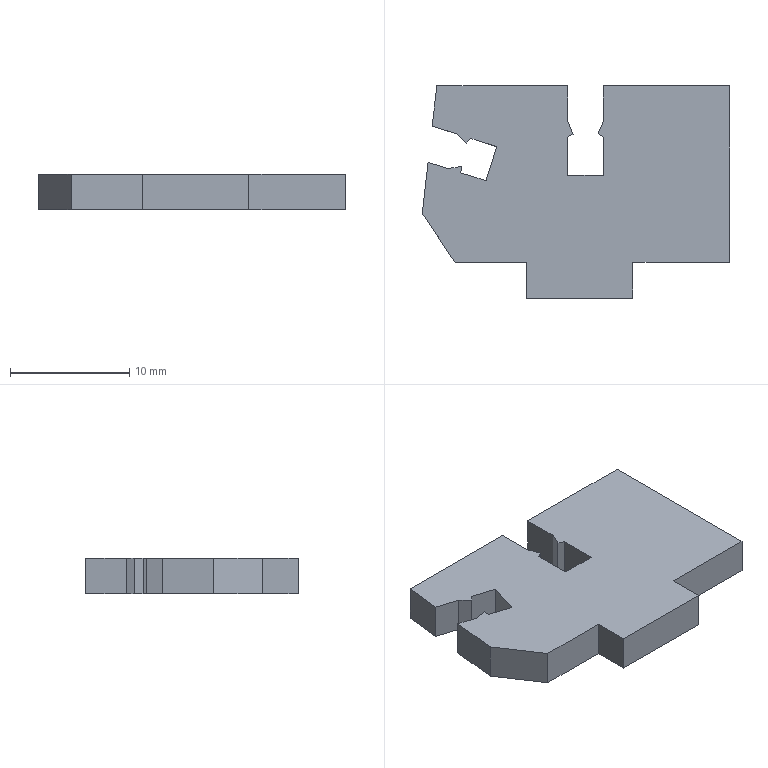Part | SolidWorks | features BaseBody 1 | 1 solid | 31 faces | box 25.767 x 17.806 x 3 mm | volume 1076 mm3 | plane 28 | spline 3
STEP:
#1=CARTESIAN_POINT('',(-24.945,11.421,-1.5));
#2=VERTEX_POINT('',#1);
#3=CARTESIAN_POINT('',(-24.55,14.81,-1.5));
#4=VERTEX_POINT('',#3);
#5=CARTESIAN_POINT('',(-24.945,11.421,-1.5));
#6=CARTESIAN_POINT('',(-24.682,13.68,-1.5));
#7=CARTESIAN_POINT('',(-24.55,14.81,-1.5));
#8=B_SPLINE_CURVE_WITH_KNOTS('',2,(#5,#6,#7),.UNSPECIFIED.,.F.,.F.,(3,3),(0.7869,0.8033),.UNSPECIFIED.);
#9=EDGE_CURVE('',#2,#4,#8,.T.);
#10=ORIENTED_EDGE('',*,*,#9,.T.);
#11=CARTESIAN_POINT('',(-13.58,14.81,-1.5));
#12=VERTEX_POINT('',#11);
#13=CARTESIAN_POINT('',(0.,14.81,-1.5));
#14=DIRECTION('',(1.,0.,0.));
#15=VECTOR('',#14,1000.);
#16=LINE('',#13,#15);
#17=EDGE_CURVE('',#4,#12,#16,.T.);
#18=ORIENTED_EDGE('',*,*,#17,.T.);
#19=CARTESIAN_POINT('',(-13.58,11.816,-1.5));
#20=VERTEX_POINT('',#19);
#21=CARTESIAN_POINT('',(-13.58,0.,-1.5));
#22=DIRECTION('',(0.,-1.,0.));
#23=VECTOR('',#22,1000.);
#24=LINE('',#21,#23);
#25=EDGE_CURVE('',#12,#20,#24,.T.);
#26=ORIENTED_EDGE('',*,*,#25,.T.);
#27=CARTESIAN_POINT('',(-13.131,10.745,-1.5));
#28=VERTEX_POINT('',#27);
#29=CARTESIAN_POINT('',(-7.343,-3.075,-1.5));
#30=DIRECTION('',(0.3863,-0.9224,0.));
#31=VECTOR('',#30,1000.);
#32=LINE('',#29,#31);
#33=EDGE_CURVE('',#20,#28,#32,.T.);
#34=ORIENTED_EDGE('',*,*,#33,.T.);
#35=CARTESIAN_POINT('',(-13.581,10.515,-1.5));
#36=VERTEX_POINT('',#35);
#37=CARTESIAN_POINT('',(-7.082,13.841,-1.5));
#38=DIRECTION('',(-0.8902,-0.4555,0.));
#39=VECTOR('',#38,1000.);
#40=LINE('',#37,#39);
#41=EDGE_CURVE('',#28,#36,#40,.T.);
#42=ORIENTED_EDGE('',*,*,#41,.T.);
#43=CARTESIAN_POINT('',(-13.583,7.301,-1.5));
#44=VERTEX_POINT('',#43);
#45=CARTESIAN_POINT('',(-13.586,0.006341,-1.5));
#46=DIRECTION('',(-0.0004667,-1.,0.));
#47=VECTOR('',#46,1000.);
#48=LINE('',#45,#47);
#49=EDGE_CURVE('',#36,#44,#48,.T.);
#50=ORIENTED_EDGE('',*,*,#49,.T.);
#51=CARTESIAN_POINT('',(-10.586,7.301,-1.5));
#52=VERTEX_POINT('',#51);
#53=CARTESIAN_POINT('',(0.,7.301,-1.5));
#54=DIRECTION('',(1.,0.,0.));
#55=VECTOR('',#54,1000.);
#56=LINE('',#53,#55);
#57=EDGE_CURVE('',#44,#52,#56,.T.);
#58=ORIENTED_EDGE('',*,*,#57,.T.);
#59=CARTESIAN_POINT('',(-10.586,10.515,-1.5));
#60=VERTEX_POINT('',#59);
#61=CARTESIAN_POINT('',(-10.586,0.,-1.5));
#62=DIRECTION('',(0.,1.,0.));
#63=VECTOR('',#62,1000.);
#64=LINE('',#61,#63);
#65=EDGE_CURVE('',#52,#60,#64,.T.);
#66=ORIENTED_EDGE('',*,*,#65,.T.);
#67=CARTESIAN_POINT('',(-11.036,10.778,-1.5));
#68=VERTEX_POINT('',#67);
#69=CARTESIAN_POINT('',(1.886,3.227,-1.5));
#70=DIRECTION('',(-0.8634,0.5045,0.));
#71=VECTOR('',#70,1000.);
#72=LINE('',#69,#71);
#73=EDGE_CURVE('',#60,#68,#72,.T.);
#74=ORIENTED_EDGE('',*,*,#73,.T.);
#75=CARTESIAN_POINT('',(-10.586,11.816,-1.5));
#76=VERTEX_POINT('',#75);
#77=CARTESIAN_POINT('',(-13.223,5.739,-1.5));
#78=DIRECTION('',(0.3981,0.9173,0.));
#79=VECTOR('',#78,1000.);
#80=LINE('',#77,#79);
#81=EDGE_CURVE('',#68,#76,#80,.T.);
#82=ORIENTED_EDGE('',*,*,#81,.T.);
#83=CARTESIAN_POINT('',(-10.588,14.81,-1.5));
#84=VERTEX_POINT('',#83);
#85=CARTESIAN_POINT('',(-10.578,-0.007066,-1.5));
#86=DIRECTION('',(-0.000668,1.,0.));
#87=VECTOR('',#86,1000.);
#88=LINE('',#85,#87);
#89=EDGE_CURVE('',#76,#84,#88,.T.);
#90=ORIENTED_EDGE('',*,*,#89,.T.);
#91=CARTESIAN_POINT('',(0.,14.81,-1.5));
#92=VERTEX_POINT('',#91);
#93=CARTESIAN_POINT('',(0.,14.81,-1.5));
#94=DIRECTION('',(1.,0.,0.));
#95=VECTOR('',#94,1000.);
#96=LINE('',#93,#95);
#97=EDGE_CURVE('',#84,#92,#96,.T.);
#98=ORIENTED_EDGE('',*,*,#97,.T.);
#99=CARTESIAN_POINT('',(0.,0.,-1.5));
#100=VERTEX_POINT('',#99);
#101=CARTESIAN_POINT('',(0.,0.,-1.5));
#102=DIRECTION('',(0.,-1.,0.));
#103=VECTOR('',#102,1000.);
#104=LINE('',#101,#103);
#105=EDGE_CURVE('',#92,#100,#104,.T.);
#106=ORIENTED_EDGE('',*,*,#105,.T.);
#107=CARTESIAN_POINT('',(-8.113,0.,-1.5));
#108=VERTEX_POINT('',#107);
#109=CARTESIAN_POINT('',(0.,0.,-1.5));
#110=DIRECTION('',(-1.,0.,0.));
#111=VECTOR('',#110,1000.);
#112=LINE('',#109,#111);
#113=EDGE_CURVE('',#100,#108,#112,.T.);
#114=ORIENTED_EDGE('',*,*,#113,.T.);
#115=CARTESIAN_POINT('',(-8.113,-2.996,-1.5));
#116=VERTEX_POINT('',#115);
#117=CARTESIAN_POINT('',(-8.113,0.,-1.5));
#118=DIRECTION('',(0.,1.,0.));
#119=VECTOR('',#118,1000.);
#120=LINE('',#117,#119);
#121=EDGE_CURVE('',#116,#108,#120,.T.);
#122=ORIENTED_EDGE('',*,*,#121,.F.);
#123=CARTESIAN_POINT('',(-17.009,-2.996,-1.5));
#124=VERTEX_POINT('',#123);
#125=CARTESIAN_POINT('',(0.,-2.996,-1.5));
#126=DIRECTION('',(-1.,0.,0.));
#127=VECTOR('',#126,1000.);
#128=LINE('',#125,#127);
#129=EDGE_CURVE('',#116,#124,#128,.T.);
#130=ORIENTED_EDGE('',*,*,#129,.T.);
#131=CARTESIAN_POINT('',(-17.009,0.,-1.5));
#132=VERTEX_POINT('',#131);
#133=CARTESIAN_POINT('',(-17.009,0.,-1.5));
#134=DIRECTION('',(0.,1.,0.));
#135=VECTOR('',#134,1000.);
#136=LINE('',#133,#135);
#137=EDGE_CURVE('',#124,#132,#136,.T.);
#138=ORIENTED_EDGE('',*,*,#137,.T.);
#139=CARTESIAN_POINT('',(-23.02,0.,-1.5));
#140=VERTEX_POINT('',#139);
#141=CARTESIAN_POINT('',(0.,0.,-1.5));
#142=DIRECTION('',(-1.,0.,0.));
#143=VECTOR('',#142,1000.);
#144=LINE('',#141,#143);
#145=EDGE_CURVE('',#132,#140,#144,.T.);
#146=ORIENTED_EDGE('',*,*,#145,.T.);
#147=CARTESIAN_POINT('',(-25.767,4.099,-1.5));
#148=VERTEX_POINT('',#147);
#149=CARTESIAN_POINT('',(-23.02,0.,-1.5));
#150=CARTESIAN_POINT('',(-23.935,1.367,-1.5));
#151=CARTESIAN_POINT('',(-24.85,2.732,-1.5));
#152=CARTESIAN_POINT('',(-25.767,4.099,-1.5));
#153=B_SPLINE_CURVE_WITH_KNOTS('',3,(#149,#150,#151,#152),.UNSPECIFIED.,.F.,.F.,(4,4),(0.6066,0.623),.UNSPECIFIED.);
#154=EDGE_CURVE('',#140,#148,#153,.T.);
#155=ORIENTED_EDGE('',*,*,#154,.T.);
#156=CARTESIAN_POINT('',(-25.29,8.389,-1.5));
#157=VERTEX_POINT('',#156);
#158=CARTESIAN_POINT('',(-25.767,4.099,-1.5));
#159=CARTESIAN_POINT('',(-25.607,5.531,-1.5));
#160=CARTESIAN_POINT('',(-25.29,8.389,-1.5));
#161=B_SPLINE_CURVE_WITH_KNOTS('',2,(#158,#159,#160),.UNSPECIFIED.,.F.,.F.,(3,3),(0.623,0.6393),.UNSPECIFIED.);
#162=EDGE_CURVE('',#148,#157,#161,.T.);
#163=ORIENTED_EDGE('',*,*,#162,.T.);
#164=CARTESIAN_POINT('',(-23.637,7.866,-1.5));
#165=VERTEX_POINT('',#164);
#166=CARTESIAN_POINT('',(0.1104,0.3489,-1.5));
#167=DIRECTION('',(0.9534,-0.3018,0.));
#168=VECTOR('',#167,1000.);
#169=LINE('',#166,#168);
#170=EDGE_CURVE('',#157,#165,#169,.T.);
#171=ORIENTED_EDGE('',*,*,#170,.T.);
#172=CARTESIAN_POINT('',(-22.501,8.049,-1.5));
#173=VERTEX_POINT('',#172);
#174=CARTESIAN_POINT('',(-1.84,11.387,-1.5));
#175=DIRECTION('',(0.9872,0.1595,0.));
#176=VECTOR('',#175,1000.);
#177=LINE('',#174,#176);
#178=EDGE_CURVE('',#165,#173,#177,.T.);
#179=ORIENTED_EDGE('',*,*,#178,.T.);
#180=CARTESIAN_POINT('',(-22.532,7.516,-1.5));
#181=VERTEX_POINT('',#180);
#182=CARTESIAN_POINT('',(-22.89,1.325,-1.5));
#183=DIRECTION('',(-0.05779,-0.9983,0.));
#184=VECTOR('',#183,1000.);
#185=LINE('',#182,#184);
#186=EDGE_CURVE('',#173,#181,#185,.T.);
#187=ORIENTED_EDGE('',*,*,#186,.T.);
#188=CARTESIAN_POINT('',(-20.425,6.852,-1.5));
#189=VERTEX_POINT('',#188);
#190=CARTESIAN_POINT('',(0.1206,0.3831,-1.5));
#191=DIRECTION('',(0.9538,-0.3003,0.));
#192=VECTOR('',#191,1000.);
#193=LINE('',#190,#192);
#194=EDGE_CURVE('',#181,#189,#193,.T.);
#195=ORIENTED_EDGE('',*,*,#194,.T.);
#196=CARTESIAN_POINT('',(-19.523,9.709,-1.5));
#197=VERTEX_POINT('',#196);
#198=CARTESIAN_POINT('',(-20.541,6.485,-1.5));
#199=DIRECTION('',(0.3011,0.9536,0.));
#200=VECTOR('',#199,1000.);
#201=LINE('',#198,#200);
#202=EDGE_CURVE('',#189,#197,#201,.T.);
#203=ORIENTED_EDGE('',*,*,#202,.T.);
#204=CARTESIAN_POINT('',(-21.692,10.394,-1.5));
#205=VERTEX_POINT('',#204);
#206=CARTESIAN_POINT('',(1.019,3.229,-1.5));
#207=DIRECTION('',(-0.9537,0.3009,0.));
#208=VECTOR('',#207,1000.);
#209=LINE('',#206,#208);
#210=EDGE_CURVE('',#197,#205,#209,.T.);
#211=ORIENTED_EDGE('',*,*,#210,.T.);
#212=CARTESIAN_POINT('',(-22.05,10.009,-1.5));
#213=VERTEX_POINT('',#212);
#214=CARTESIAN_POINT('',(-16.776,15.659,-1.5));
#215=DIRECTION('',(-0.6824,-0.731,0.));
#216=VECTOR('',#215,1000.);
#217=LINE('',#214,#216);
#218=EDGE_CURVE('',#205,#213,#217,.T.);
#219=ORIENTED_EDGE('',*,*,#218,.T.);
#220=CARTESIAN_POINT('',(-22.83,10.752,-1.5));
#221=VERTEX_POINT('',#220);
#222=CARTESIAN_POINT('',(-5.502,-5.77,-1.5));
#223=DIRECTION('',(-0.7237,0.6901,0.));
#224=VECTOR('',#223,1000.);
#225=LINE('',#222,#224);
#226=EDGE_CURVE('',#213,#221,#225,.T.);
#227=ORIENTED_EDGE('',*,*,#226,.T.);
#228=CARTESIAN_POINT('',(1.015,3.211,-1.5));
#229=DIRECTION('',(-0.9535,0.3015,0.));
#230=VECTOR('',#229,1000.);
#231=LINE('',#228,#230);
#232=EDGE_CURVE('',#221,#2,#231,.T.);
#233=ORIENTED_EDGE('',*,*,#232,.T.);
#234=EDGE_LOOP('',(#10,#18,#26,#34,#42,#50,#58,#66,#74,#82,#90,#98,#106,#114,#122,#130,#138,#146,#155,#163,#171,#179,#187,#195,#203,#211,#219,#227,#233));
#235=FACE_OUTER_BOUND('',#234,.T.);
#236=CARTESIAN_POINT('',(0.,0.,-1.5));
#237=DIRECTION('',(0.,0.,1.));
#238=DIRECTION('',(1.,0.,0.));
#239=AXIS2_PLACEMENT_3D('',#236,#237,#238);
#240=PLANE('',#239);
#241=ADVANCED_FACE('',(#235),#240,.F.);
#242=CARTESIAN_POINT('',(-24.945,11.421,1.5));
#243=VERTEX_POINT('',#242);
#244=CARTESIAN_POINT('',(-24.55,14.81,1.5));
#245=VERTEX_POINT('',#244);
#246=CARTESIAN_POINT('',(-24.945,11.421,1.5));
#247=CARTESIAN_POINT('',(-24.682,13.68,1.5));
#248=CARTESIAN_POINT('',(-24.55,14.81,1.5));
#249=B_SPLINE_CURVE_WITH_KNOTS('',2,(#246,#247,#248),.UNSPECIFIED.,.F.,.F.,(3,3),(0.7869,0.8033),.UNSPECIFIED.);
#250=EDGE_CURVE('',#243,#245,#249,.T.);
#251=ORIENTED_EDGE('',*,*,#250,.F.);
#252=CARTESIAN_POINT('',(-22.83,10.752,1.5));
#253=VERTEX_POINT('',#252);
#254=CARTESIAN_POINT('',(1.015,3.211,1.5));
#255=DIRECTION('',(-0.9535,0.3015,0.));
#256=VECTOR('',#255,1000.);
#257=LINE('',#254,#256);
#258=EDGE_CURVE('',#253,#243,#257,.T.);
#259=ORIENTED_EDGE('',*,*,#258,.F.);
#260=CARTESIAN_POINT('',(-22.05,10.009,1.5));
#261=VERTEX_POINT('',#260);
#262=CARTESIAN_POINT('',(-5.502,-5.77,1.5));
#263=DIRECTION('',(-0.7237,0.6901,0.));
#264=VECTOR('',#263,1000.);
#265=LINE('',#262,#264);
#266=EDGE_CURVE('',#261,#253,#265,.T.);
#267=ORIENTED_EDGE('',*,*,#266,.F.);
#268=CARTESIAN_POINT('',(-21.692,10.394,1.5));
#269=VERTEX_POINT('',#268);
#270=CARTESIAN_POINT('',(-16.776,15.659,1.5));
#271=DIRECTION('',(-0.6824,-0.731,0.));
#272=VECTOR('',#271,1000.);
#273=LINE('',#270,#272);
#274=EDGE_CURVE('',#269,#261,#273,.T.);
#275=ORIENTED_EDGE('',*,*,#274,.F.);
#276=CARTESIAN_POINT('',(-19.523,9.709,1.5));
#277=VERTEX_POINT('',#276);
#278=CARTESIAN_POINT('',(1.019,3.229,1.5));
#279=DIRECTION('',(-0.9537,0.3009,0.));
#280=VECTOR('',#279,1000.);
#281=LINE('',#278,#280);
#282=EDGE_CURVE('',#277,#269,#281,.T.);
#283=ORIENTED_EDGE('',*,*,#282,.F.);
#284=CARTESIAN_POINT('',(-20.425,6.852,1.5));
#285=VERTEX_POINT('',#284);
#286=CARTESIAN_POINT('',(-20.541,6.485,1.5));
#287=DIRECTION('',(0.3011,0.9536,0.));
#288=VECTOR('',#287,1000.);
#289=LINE('',#286,#288);
#290=EDGE_CURVE('',#285,#277,#289,.T.);
#291=ORIENTED_EDGE('',*,*,#290,.F.);
#292=CARTESIAN_POINT('',(-22.532,7.516,1.5));
#293=VERTEX_POINT('',#292);
#294=CARTESIAN_POINT('',(0.1206,0.3831,1.5));
#295=DIRECTION('',(0.9538,-0.3003,0.));
#296=VECTOR('',#295,1000.);
#297=LINE('',#294,#296);
#298=EDGE_CURVE('',#293,#285,#297,.T.);
#299=ORIENTED_EDGE('',*,*,#298,.F.);
#300=CARTESIAN_POINT('',(-22.501,8.049,1.5));
#301=VERTEX_POINT('',#300);
#302=CARTESIAN_POINT('',(-22.89,1.325,1.5));
#303=DIRECTION('',(-0.05779,-0.9983,0.));
#304=VECTOR('',#303,1000.);
#305=LINE('',#302,#304);
#306=EDGE_CURVE('',#301,#293,#305,.T.);
#307=ORIENTED_EDGE('',*,*,#306,.F.);
#308=CARTESIAN_POINT('',(-23.637,7.866,1.5));
#309=VERTEX_POINT('',#308);
#310=CARTESIAN_POINT('',(-1.84,11.387,1.5));
#311=DIRECTION('',(0.9872,0.1595,0.));
#312=VECTOR('',#311,1000.);
#313=LINE('',#310,#312);
#314=EDGE_CURVE('',#309,#301,#313,.T.);
#315=ORIENTED_EDGE('',*,*,#314,.F.);
#316=CARTESIAN_POINT('',(-25.29,8.389,1.5));
#317=VERTEX_POINT('',#316);
#318=CARTESIAN_POINT('',(0.1104,0.3489,1.5));
#319=DIRECTION('',(0.9534,-0.3018,0.));
#320=VECTOR('',#319,1000.);
#321=LINE('',#318,#320);
#322=EDGE_CURVE('',#317,#309,#321,.T.);
#323=ORIENTED_EDGE('',*,*,#322,.F.);
#324=CARTESIAN_POINT('',(-25.767,4.099,1.5));
#325=VERTEX_POINT('',#324);
#326=CARTESIAN_POINT('',(-25.767,4.099,1.5));
#327=CARTESIAN_POINT('',(-25.607,5.531,1.5));
#328=CARTESIAN_POINT('',(-25.29,8.389,1.5));
#329=B_SPLINE_CURVE_WITH_KNOTS('',2,(#326,#327,#328),.UNSPECIFIED.,.F.,.F.,(3,3),(0.623,0.6393),.UNSPECIFIED.);
#330=EDGE_CURVE('',#325,#317,#329,.T.);
#331=ORIENTED_EDGE('',*,*,#330,.F.);
#332=CARTESIAN_POINT('',(-23.02,0.,1.5));
#333=VERTEX_POINT('',#332);
#334=CARTESIAN_POINT('',(-23.02,0.,1.5));
#335=CARTESIAN_POINT('',(-23.935,1.367,1.5));
#336=CARTESIAN_POINT('',(-24.85,2.732,1.5));
#337=CARTESIAN_POINT('',(-25.767,4.099,1.5));
#338=B_SPLINE_CURVE_WITH_KNOTS('',3,(#334,#335,#336,#337),.UNSPECIFIED.,.F.,.F.,(4,4),(0.6066,0.623),.UNSPECIFIED.);
#339=EDGE_CURVE('',#333,#325,#338,.T.);
#340=ORIENTED_EDGE('',*,*,#339,.F.);
#341=CARTESIAN_POINT('',(-17.009,0.,1.5));
#342=VERTEX_POINT('',#341);
#343=CARTESIAN_POINT('',(0.,0.,1.5));
#344=DIRECTION('',(-1.,0.,0.));
#345=VECTOR('',#344,1000.);
#346=LINE('',#343,#345);
#347=EDGE_CURVE('',#342,#333,#346,.T.);
#348=ORIENTED_EDGE('',*,*,#347,.F.);
#349=CARTESIAN_POINT('',(-17.009,-2.996,1.5));
#350=VERTEX_POINT('',#349);
#351=CARTESIAN_POINT('',(-17.009,0.,1.5));
#352=DIRECTION('',(0.,1.,0.));
#353=VECTOR('',#352,1000.);
#354=LINE('',#351,#353);
#355=EDGE_CURVE('',#350,#342,#354,.T.);
#356=ORIENTED_EDGE('',*,*,#355,.F.);
#357=CARTESIAN_POINT('',(-8.113,-2.996,1.5));
#358=VERTEX_POINT('',#357);
#359=CARTESIAN_POINT('',(0.,-2.996,1.5));
#360=DIRECTION('',(-1.,0.,0.));
#361=VECTOR('',#360,1000.);
#362=LINE('',#359,#361);
#363=EDGE_CURVE('',#358,#350,#362,.T.);
#364=ORIENTED_EDGE('',*,*,#363,.F.);
#365=CARTESIAN_POINT('',(-8.113,0.,1.5));
#366=VERTEX_POINT('',#365);
#367=CARTESIAN_POINT('',(-8.113,0.,1.5));
#368=DIRECTION('',(0.,1.,0.));
#369=VECTOR('',#368,1000.);
#370=LINE('',#367,#369);
#371=EDGE_CURVE('',#358,#366,#370,.T.);
#372=ORIENTED_EDGE('',*,*,#371,.T.);
#373=CARTESIAN_POINT('',(0.,0.,1.5));
#374=VERTEX_POINT('',#373);
#375=CARTESIAN_POINT('',(0.,0.,1.5));
#376=DIRECTION('',(-1.,0.,0.));
#377=VECTOR('',#376,1000.);
#378=LINE('',#375,#377);
#379=EDGE_CURVE('',#374,#366,#378,.T.);
#380=ORIENTED_EDGE('',*,*,#379,.F.);
#381=CARTESIAN_POINT('',(0.,14.81,1.5));
#382=VERTEX_POINT('',#381);
#383=CARTESIAN_POINT('',(0.,0.,1.5));
#384=DIRECTION('',(0.,-1.,0.));
#385=VECTOR('',#384,1000.);
#386=LINE('',#383,#385);
#387=EDGE_CURVE('',#382,#374,#386,.T.);
#388=ORIENTED_EDGE('',*,*,#387,.F.);
#389=CARTESIAN_POINT('',(-10.588,14.81,1.5));
#390=VERTEX_POINT('',#389);
#391=CARTESIAN_POINT('',(0.,14.81,1.5));
#392=DIRECTION('',(1.,0.,0.));
#393=VECTOR('',#392,1000.);
#394=LINE('',#391,#393);
#395=EDGE_CURVE('',#390,#382,#394,.T.);
#396=ORIENTED_EDGE('',*,*,#395,.F.);
#397=CARTESIAN_POINT('',(-10.586,11.816,1.5));
#398=VERTEX_POINT('',#397);
#399=CARTESIAN_POINT('',(-10.578,-0.007066,1.5));
#400=DIRECTION('',(-0.000668,1.,0.));
#401=VECTOR('',#400,1000.);
#402=LINE('',#399,#401);
#403=EDGE_CURVE('',#398,#390,#402,.T.);
#404=ORIENTED_EDGE('',*,*,#403,.F.);
#405=CARTESIAN_POINT('',(-11.036,10.778,1.5));
#406=VERTEX_POINT('',#405);
#407=CARTESIAN_POINT('',(-13.223,5.739,1.5));
#408=DIRECTION('',(0.3981,0.9173,0.));
#409=VECTOR('',#408,1000.);
#410=LINE('',#407,#409);
#411=EDGE_CURVE('',#406,#398,#410,.T.);
#412=ORIENTED_EDGE('',*,*,#411,.F.);
#413=CARTESIAN_POINT('',(-10.586,10.515,1.5));
#414=VERTEX_POINT('',#413);
#415=CARTESIAN_POINT('',(1.886,3.227,1.5));
#416=DIRECTION('',(-0.8634,0.5045,0.));
#417=VECTOR('',#416,1000.);
#418=LINE('',#415,#417);
#419=EDGE_CURVE('',#414,#406,#418,.T.);
#420=ORIENTED_EDGE('',*,*,#419,.F.);
#421=CARTESIAN_POINT('',(-10.586,7.301,1.5));
#422=VERTEX_POINT('',#421);
#423=CARTESIAN_POINT('',(-10.586,0.,1.5));
#424=DIRECTION('',(0.,1.,0.));
#425=VECTOR('',#424,1000.);
#426=LINE('',#423,#425);
#427=EDGE_CURVE('',#422,#414,#426,.T.);
#428=ORIENTED_EDGE('',*,*,#427,.F.);
#429=CARTESIAN_POINT('',(-13.583,7.301,1.5));
#430=VERTEX_POINT('',#429);
#431=CARTESIAN_POINT('',(0.,7.301,1.5));
#432=DIRECTION('',(1.,0.,0.));
#433=VECTOR('',#432,1000.);
#434=LINE('',#431,#433);
#435=EDGE_CURVE('',#430,#422,#434,.T.);
#436=ORIENTED_EDGE('',*,*,#435,.F.);
#437=CARTESIAN_POINT('',(-13.581,10.515,1.5));
#438=VERTEX_POINT('',#437);
#439=CARTESIAN_POINT('',(-13.586,0.006341,1.5));
#440=DIRECTION('',(-0.0004667,-1.,0.));
#441=VECTOR('',#440,1000.);
#442=LINE('',#439,#441);
#443=EDGE_CURVE('',#438,#430,#442,.T.);
#444=ORIENTED_EDGE('',*,*,#443,.F.);
#445=CARTESIAN_POINT('',(-13.131,10.745,1.5));
#446=VERTEX_POINT('',#445);
#447=CARTESIAN_POINT('',(-7.082,13.841,1.5));
#448=DIRECTION('',(-0.8902,-0.4555,0.));
#449=VECTOR('',#448,1000.);
#450=LINE('',#447,#449);
#451=EDGE_CURVE('',#446,#438,#450,.T.);
#452=ORIENTED_EDGE('',*,*,#451,.F.);
#453=CARTESIAN_POINT('',(-13.58,11.816,1.5));
#454=VERTEX_POINT('',#453);
#455=CARTESIAN_POINT('',(-7.343,-3.075,1.5));
#456=DIRECTION('',(0.3863,-0.9224,0.));
#457=VECTOR('',#456,1000.);
#458=LINE('',#455,#457);
#459=EDGE_CURVE('',#454,#446,#458,.T.);
#460=ORIENTED_EDGE('',*,*,#459,.F.);
#461=CARTESIAN_POINT('',(-13.58,14.81,1.5));
#462=VERTEX_POINT('',#461);
#463=CARTESIAN_POINT('',(-13.58,0.,1.5));
#464=DIRECTION('',(0.,-1.,0.));
#465=VECTOR('',#464,1000.);
#466=LINE('',#463,#465);
#467=EDGE_CURVE('',#462,#454,#466,.T.);
#468=ORIENTED_EDGE('',*,*,#467,.F.);
#469=CARTESIAN_POINT('',(0.,14.81,1.5));
#470=DIRECTION('',(1.,0.,0.));
#471=VECTOR('',#470,1000.);
#472=LINE('',#469,#471);
#473=EDGE_CURVE('',#245,#462,#472,.T.);
#474=ORIENTED_EDGE('',*,*,#473,.F.);
#475=EDGE_LOOP('',(#251,#259,#267,#275,#283,#291,#299,#307,#315,#323,#331,#340,#348,#356,#364,#372,#380,#388,#396,#404,#412,#420,#428,#436,#444,#452,#460,#468,#474));
#476=FACE_OUTER_BOUND('',#475,.T.);
#477=CARTESIAN_POINT('',(0.,0.,1.5));
#478=DIRECTION('',(0.,0.,1.));
#479=DIRECTION('',(1.,0.,0.));
#480=AXIS2_PLACEMENT_3D('',#477,#478,#479);
#481=PLANE('',#480);
#482=ADVANCED_FACE('',(#476),#481,.T.);
#483=ORIENTED_EDGE('',*,*,#17,.F.);
#484=CARTESIAN_POINT('',(-24.55,14.81,1.5));
#485=DIRECTION('',(0.,0.,-1.));
#486=VECTOR('',#485,1000.);
#487=LINE('',#484,#486);
#488=EDGE_CURVE('',#245,#4,#487,.T.);
#489=ORIENTED_EDGE('',*,*,#488,.F.);
#490=ORIENTED_EDGE('',*,*,#473,.T.);
#491=CARTESIAN_POINT('',(-13.58,14.81,1.5));
#492=DIRECTION('',(0.,0.,-1.));
#493=VECTOR('',#492,1000.);
#494=LINE('',#491,#493);
#495=EDGE_CURVE('',#462,#12,#494,.T.);
#496=ORIENTED_EDGE('',*,*,#495,.T.);
#497=EDGE_LOOP('',(#483,#489,#490,#496));
#498=FACE_OUTER_BOUND('',#497,.T.);
#499=CARTESIAN_POINT('',(0.,14.81,1.5));
#500=DIRECTION('',(0.,1.,0.));
#501=DIRECTION('',(1.,0.,0.));
#502=AXIS2_PLACEMENT_3D('',#499,#500,#501);
#503=PLANE('',#502);
#504=ADVANCED_FACE('',(#498),#503,.T.);
#505=ORIENTED_EDGE('',*,*,#25,.F.);
#506=ORIENTED_EDGE('',*,*,#495,.F.);
#507=ORIENTED_EDGE('',*,*,#467,.T.);
#508=CARTESIAN_POINT('',(-13.58,11.816,1.5));
#509=DIRECTION('',(0.,0.,-1.));
#510=VECTOR('',#509,1000.);
#511=LINE('',#508,#510);
#512=EDGE_CURVE('',#454,#20,#511,.T.);
#513=ORIENTED_EDGE('',*,*,#512,.T.);
#514=EDGE_LOOP('',(#505,#506,#507,#513));
#515=FACE_OUTER_BOUND('',#514,.T.);
#516=CARTESIAN_POINT('',(-13.58,0.,1.5));
#517=DIRECTION('',(1.,0.,0.));
#518=DIRECTION('',(0.,1.,0.));
#519=AXIS2_PLACEMENT_3D('',#516,#517,#518);
#520=PLANE('',#519);
#521=ADVANCED_FACE('',(#515),#520,.T.);
#522=ORIENTED_EDGE('',*,*,#33,.F.);
#523=ORIENTED_EDGE('',*,*,#512,.F.);
#524=ORIENTED_EDGE('',*,*,#459,.T.);
#525=CARTESIAN_POINT('',(-13.131,10.745,1.5));
#526=DIRECTION('',(0.,0.,-1.));
#527=VECTOR('',#526,1000.);
#528=LINE('',#525,#527);
#529=EDGE_CURVE('',#446,#28,#528,.T.);
#530=ORIENTED_EDGE('',*,*,#529,.T.);
#531=EDGE_LOOP('',(#522,#523,#524,#530));
#532=FACE_OUTER_BOUND('',#531,.T.);
#533=CARTESIAN_POINT('',(-7.343,-3.075,1.5));
#534=DIRECTION('',(0.9224,0.3863,0.));
#535=DIRECTION('',(0.,0.,-1.));
#536=AXIS2_PLACEMENT_3D('',#533,#534,#535);
#537=PLANE('',#536);
#538=ADVANCED_FACE('',(#532),#537,.T.);
#539=ORIENTED_EDGE('',*,*,#41,.F.);
#540=ORIENTED_EDGE('',*,*,#529,.F.);
#541=ORIENTED_EDGE('',*,*,#451,.T.);
#542=CARTESIAN_POINT('',(-13.581,10.515,1.5));
#543=DIRECTION('',(0.,0.,-1.));
#544=VECTOR('',#543,1000.);
#545=LINE('',#542,#544);
#546=EDGE_CURVE('',#438,#36,#545,.T.);
#547=ORIENTED_EDGE('',*,*,#546,.T.);
#548=EDGE_LOOP('',(#539,#540,#541,#547));
#549=FACE_OUTER_BOUND('',#548,.T.);
#550=CARTESIAN_POINT('',(-7.082,13.841,1.5));
#551=DIRECTION('',(0.4555,-0.8902,0.));
#552=DIRECTION('',(0.,0.,-1.));
#553=AXIS2_PLACEMENT_3D('',#550,#551,#552);
#554=PLANE('',#553);
#555=ADVANCED_FACE('',(#549),#554,.T.);
#556=ORIENTED_EDGE('',*,*,#49,.F.);
#557=ORIENTED_EDGE('',*,*,#546,.F.);
#558=ORIENTED_EDGE('',*,*,#443,.T.);
#559=CARTESIAN_POINT('',(-13.583,7.301,1.5));
#560=DIRECTION('',(0.,0.,-1.));
#561=VECTOR('',#560,1000.);
#562=LINE('',#559,#561);
#563=EDGE_CURVE('',#430,#44,#562,.T.);
#564=ORIENTED_EDGE('',*,*,#563,.T.);
#565=EDGE_LOOP('',(#556,#557,#558,#564));
#566=FACE_OUTER_BOUND('',#565,.T.);
#567=CARTESIAN_POINT('',(-13.586,0.006341,1.5));
#568=DIRECTION('',(1.,-0.0004667,0.));
#569=DIRECTION('',(0.,0.,-1.));
#570=AXIS2_PLACEMENT_3D('',#567,#568,#569);
#571=PLANE('',#570);
#572=ADVANCED_FACE('',(#566),#571,.T.);
#573=ORIENTED_EDGE('',*,*,#57,.F.);
#574=ORIENTED_EDGE('',*,*,#563,.F.);
#575=ORIENTED_EDGE('',*,*,#435,.T.);
#576=CARTESIAN_POINT('',(-10.586,7.301,1.5));
#577=DIRECTION('',(0.,0.,-1.));
#578=VECTOR('',#577,1000.);
#579=LINE('',#576,#578);
#580=EDGE_CURVE('',#422,#52,#579,.T.);
#581=ORIENTED_EDGE('',*,*,#580,.T.);
#582=EDGE_LOOP('',(#573,#574,#575,#581));
#583=FACE_OUTER_BOUND('',#582,.T.);
#584=CARTESIAN_POINT('',(0.,7.301,1.5));
#585=DIRECTION('',(0.,1.,0.));
#586=DIRECTION('',(1.,0.,0.));
#587=AXIS2_PLACEMENT_3D('',#584,#585,#586);
#588=PLANE('',#587);
#589=ADVANCED_FACE('',(#583),#588,.T.);
#590=ORIENTED_EDGE('',*,*,#65,.F.);
#591=ORIENTED_EDGE('',*,*,#580,.F.);
#592=ORIENTED_EDGE('',*,*,#427,.T.);
#593=CARTESIAN_POINT('',(-10.586,10.515,1.5));
#594=DIRECTION('',(0.,0.,-1.));
#595=VECTOR('',#594,1000.);
#596=LINE('',#593,#595);
#597=EDGE_CURVE('',#414,#60,#596,.T.);
#598=ORIENTED_EDGE('',*,*,#597,.T.);
#599=EDGE_LOOP('',(#590,#591,#592,#598));
#600=FACE_OUTER_BOUND('',#599,.T.);
#601=CARTESIAN_POINT('',(-10.586,0.,1.5));
#602=DIRECTION('',(-1.,0.,0.));
#603=DIRECTION('',(0.,0.,1.));
#604=AXIS2_PLACEMENT_3D('',#601,#602,#603);
#605=PLANE('',#604);
#606=ADVANCED_FACE('',(#600),#605,.T.);
#607=ORIENTED_EDGE('',*,*,#73,.F.);
#608=ORIENTED_EDGE('',*,*,#597,.F.);
#609=ORIENTED_EDGE('',*,*,#419,.T.);
#610=CARTESIAN_POINT('',(-11.036,10.778,1.5));
#611=DIRECTION('',(0.,0.,-1.));
#612=VECTOR('',#611,1000.);
#613=LINE('',#610,#612);
#614=EDGE_CURVE('',#406,#68,#613,.T.);
#615=ORIENTED_EDGE('',*,*,#614,.T.);
#616=EDGE_LOOP('',(#607,#608,#609,#615));
#617=FACE_OUTER_BOUND('',#616,.T.);
#618=CARTESIAN_POINT('',(1.886,3.227,1.5));
#619=DIRECTION('',(-0.5045,-0.8634,0.));
#620=DIRECTION('',(-0.8634,0.5045,0.));
#621=AXIS2_PLACEMENT_3D('',#618,#619,#620);
#622=PLANE('',#621);
#623=ADVANCED_FACE('',(#617),#622,.T.);
#624=ORIENTED_EDGE('',*,*,#81,.F.);
#625=ORIENTED_EDGE('',*,*,#614,.F.);
#626=ORIENTED_EDGE('',*,*,#411,.T.);
#627=CARTESIAN_POINT('',(-10.586,11.816,1.5));
#628=DIRECTION('',(0.,0.,-1.));
#629=VECTOR('',#628,1000.);
#630=LINE('',#627,#629);
#631=EDGE_CURVE('',#398,#76,#630,.T.);
#632=ORIENTED_EDGE('',*,*,#631,.T.);
#633=EDGE_LOOP('',(#624,#625,#626,#632));
#634=FACE_OUTER_BOUND('',#633,.T.);
#635=CARTESIAN_POINT('',(-13.223,5.739,1.5));
#636=DIRECTION('',(-0.9173,0.3981,0.));
#637=DIRECTION('',(0.,0.,1.));
#638=AXIS2_PLACEMENT_3D('',#635,#636,#637);
#639=PLANE('',#638);
#640=ADVANCED_FACE('',(#634),#639,.T.);
#641=ORIENTED_EDGE('',*,*,#89,.F.);
#642=ORIENTED_EDGE('',*,*,#631,.F.);
#643=ORIENTED_EDGE('',*,*,#403,.T.);
#644=CARTESIAN_POINT('',(-10.588,14.81,1.5));
#645=DIRECTION('',(0.,0.,-1.));
#646=VECTOR('',#645,1000.);
#647=LINE('',#644,#646);
#648=EDGE_CURVE('',#390,#84,#647,.T.);
#649=ORIENTED_EDGE('',*,*,#648,.T.);
#650=EDGE_LOOP('',(#641,#642,#643,#649));
#651=FACE_OUTER_BOUND('',#650,.T.);
#652=CARTESIAN_POINT('',(-10.578,-0.007066,1.5));
#653=DIRECTION('',(-1.,-0.000668,0.));
#654=DIRECTION('',(-0.000668,1.,0.));
#655=AXIS2_PLACEMENT_3D('',#652,#653,#654);
#656=PLANE('',#655);
#657=ADVANCED_FACE('',(#651),#656,.T.);
#658=ORIENTED_EDGE('',*,*,#97,.F.);
#659=ORIENTED_EDGE('',*,*,#648,.F.);
#660=ORIENTED_EDGE('',*,*,#395,.T.);
#661=CARTESIAN_POINT('',(0.,14.81,1.5));
#662=DIRECTION('',(0.,0.,-1.));
#663=VECTOR('',#662,1000.);
#664=LINE('',#661,#663);
#665=EDGE_CURVE('',#382,#92,#664,.T.);
#666=ORIENTED_EDGE('',*,*,#665,.T.);
#667=EDGE_LOOP('',(#658,#659,#660,#666));
#668=FACE_OUTER_BOUND('',#667,.T.);
#669=CARTESIAN_POINT('',(0.,14.81,1.5));
#670=DIRECTION('',(0.,1.,0.));
#671=DIRECTION('',(1.,0.,0.));
#672=AXIS2_PLACEMENT_3D('',#669,#670,#671);
#673=PLANE('',#672);
#674=ADVANCED_FACE('',(#668),#673,.T.);
#675=ORIENTED_EDGE('',*,*,#105,.F.);
#676=ORIENTED_EDGE('',*,*,#665,.F.);
#677=ORIENTED_EDGE('',*,*,#387,.T.);
#678=CARTESIAN_POINT('',(0.,0.,1.5));
#679=DIRECTION('',(0.,0.,-1.));
#680=VECTOR('',#679,1000.);
#681=LINE('',#678,#680);
#682=EDGE_CURVE('',#374,#100,#681,.T.);
#683=ORIENTED_EDGE('',*,*,#682,.T.);
#684=EDGE_LOOP('',(#675,#676,#677,#683));
#685=FACE_OUTER_BOUND('',#684,.T.);
#686=CARTESIAN_POINT('',(0.,0.,1.5));
#687=DIRECTION('',(1.,0.,0.));
#688=DIRECTION('',(0.,1.,0.));
#689=AXIS2_PLACEMENT_3D('',#686,#687,#688);
#690=PLANE('',#689);
#691=ADVANCED_FACE('',(#685),#690,.T.);
#692=ORIENTED_EDGE('',*,*,#113,.F.);
#693=ORIENTED_EDGE('',*,*,#682,.F.);
#694=ORIENTED_EDGE('',*,*,#379,.T.);
#695=CARTESIAN_POINT('',(-8.113,0.,1.5));
#696=DIRECTION('',(0.,0.,-1.));
#697=VECTOR('',#696,1000.);
#698=LINE('',#695,#697);
#699=EDGE_CURVE('',#366,#108,#698,.T.);
#700=ORIENTED_EDGE('',*,*,#699,.T.);
#701=EDGE_LOOP('',(#692,#693,#694,#700));
#702=FACE_OUTER_BOUND('',#701,.T.);
#703=CARTESIAN_POINT('',(0.,0.,1.5));
#704=DIRECTION('',(0.,-1.,0.));
#705=DIRECTION('',(0.,0.,-1.));
#706=AXIS2_PLACEMENT_3D('',#703,#704,#705);
#707=PLANE('',#706);
#708=ADVANCED_FACE('',(#702),#707,.T.);
#709=ORIENTED_EDGE('',*,*,#121,.T.);
#710=ORIENTED_EDGE('',*,*,#699,.F.);
#711=ORIENTED_EDGE('',*,*,#371,.F.);
#712=CARTESIAN_POINT('',(-8.113,-2.996,1.5));
#713=DIRECTION('',(0.,0.,-1.));
#714=VECTOR('',#713,1000.);
#715=LINE('',#712,#714);
#716=EDGE_CURVE('',#358,#116,#715,.T.);
#717=ORIENTED_EDGE('',*,*,#716,.T.);
#718=EDGE_LOOP('',(#709,#710,#711,#717));
#719=FACE_OUTER_BOUND('',#718,.T.);
#720=CARTESIAN_POINT('',(-8.113,0.,1.5));
#721=DIRECTION('',(-1.,0.,0.));
#722=DIRECTION('',(0.,0.,1.));
#723=AXIS2_PLACEMENT_3D('',#720,#721,#722);
#724=PLANE('',#723);
#725=ADVANCED_FACE('',(#719),#724,.F.);
#726=ORIENTED_EDGE('',*,*,#129,.F.);
#727=ORIENTED_EDGE('',*,*,#716,.F.);
#728=ORIENTED_EDGE('',*,*,#363,.T.);
#729=CARTESIAN_POINT('',(-17.009,-2.996,1.5));
#730=DIRECTION('',(0.,0.,-1.));
#731=VECTOR('',#730,1000.);
#732=LINE('',#729,#731);
#733=EDGE_CURVE('',#350,#124,#732,.T.);
#734=ORIENTED_EDGE('',*,*,#733,.T.);
#735=EDGE_LOOP('',(#726,#727,#728,#734));
#736=FACE_OUTER_BOUND('',#735,.T.);
#737=CARTESIAN_POINT('',(0.,-2.996,1.5));
#738=DIRECTION('',(0.,-1.,0.));
#739=DIRECTION('',(0.,0.,-1.));
#740=AXIS2_PLACEMENT_3D('',#737,#738,#739);
#741=PLANE('',#740);
#742=ADVANCED_FACE('',(#736),#741,.T.);
#743=ORIENTED_EDGE('',*,*,#137,.F.);
#744=ORIENTED_EDGE('',*,*,#733,.F.);
#745=ORIENTED_EDGE('',*,*,#355,.T.);
#746=CARTESIAN_POINT('',(-17.009,0.,1.5));
#747=DIRECTION('',(0.,0.,-1.));
#748=VECTOR('',#747,1000.);
#749=LINE('',#746,#748);
#750=EDGE_CURVE('',#342,#132,#749,.T.);
#751=ORIENTED_EDGE('',*,*,#750,.T.);
#752=EDGE_LOOP('',(#743,#744,#745,#751));
#753=FACE_OUTER_BOUND('',#752,.T.);
#754=CARTESIAN_POINT('',(-17.009,0.,1.5));
#755=DIRECTION('',(-1.,0.,0.));
#756=DIRECTION('',(0.,0.,1.));
#757=AXIS2_PLACEMENT_3D('',#754,#755,#756);
#758=PLANE('',#757);
#759=ADVANCED_FACE('',(#753),#758,.T.);
#760=ORIENTED_EDGE('',*,*,#145,.F.);
#761=ORIENTED_EDGE('',*,*,#750,.F.);
#762=ORIENTED_EDGE('',*,*,#347,.T.);
#763=CARTESIAN_POINT('',(-23.02,0.,1.5));
#764=DIRECTION('',(0.,0.,-1.));
#765=VECTOR('',#764,1000.);
#766=LINE('',#763,#765);
#767=EDGE_CURVE('',#333,#140,#766,.T.);
#768=ORIENTED_EDGE('',*,*,#767,.T.);
#769=EDGE_LOOP('',(#760,#761,#762,#768));
#770=FACE_OUTER_BOUND('',#769,.T.);
#771=CARTESIAN_POINT('',(0.,0.,1.5));
#772=DIRECTION('',(0.,-1.,0.));
#773=DIRECTION('',(0.,0.,-1.));
#774=AXIS2_PLACEMENT_3D('',#771,#772,#773);
#775=PLANE('',#774);
#776=ADVANCED_FACE('',(#770),#775,.T.);
#777=ORIENTED_EDGE('',*,*,#154,.F.);
#778=ORIENTED_EDGE('',*,*,#767,.F.);
#779=ORIENTED_EDGE('',*,*,#339,.T.);
#780=CARTESIAN_POINT('',(-25.767,4.099,1.5));
#781=DIRECTION('',(0.,0.,-1.));
#782=VECTOR('',#781,1000.);
#783=LINE('',#780,#782);
#784=EDGE_CURVE('',#325,#148,#783,.T.);
#785=ORIENTED_EDGE('',*,*,#784,.T.);
#786=EDGE_LOOP('',(#777,#778,#779,#785));
#787=FACE_OUTER_BOUND('',#786,.T.);
#788=CARTESIAN_POINT('',(-23.02,0.,1.5));
#789=CARTESIAN_POINT('',(-23.02,0.,-1.5));
#790=CARTESIAN_POINT('',(-23.935,1.367,1.5));
#791=CARTESIAN_POINT('',(-23.935,1.367,-1.5));
#792=CARTESIAN_POINT('',(-24.85,2.732,1.5));
#793=CARTESIAN_POINT('',(-24.85,2.732,-1.5));
#794=CARTESIAN_POINT('',(-25.767,4.099,1.5));
#795=CARTESIAN_POINT('',(-25.767,4.099,-1.5));
#796=B_SPLINE_SURFACE_WITH_KNOTS('',3,1,((#788,#789),(#790,#791),(#792,#793),(#794,#795)),.UNSPECIFIED.,.F.,.F.,.F.,(4,4),(2,2),(0.6066,0.623),(0.,1.),.UNSPECIFIED.);
#797=ADVANCED_FACE('',(#787),#796,.T.);
#798=ORIENTED_EDGE('',*,*,#162,.F.);
#799=ORIENTED_EDGE('',*,*,#784,.F.);
#800=ORIENTED_EDGE('',*,*,#330,.T.);
#801=CARTESIAN_POINT('',(-25.29,8.389,1.5));
#802=DIRECTION('',(0.,0.,-1.));
#803=VECTOR('',#802,1000.);
#804=LINE('',#801,#803);
#805=EDGE_CURVE('',#317,#157,#804,.T.);
#806=ORIENTED_EDGE('',*,*,#805,.T.);
#807=EDGE_LOOP('',(#798,#799,#800,#806));
#808=FACE_OUTER_BOUND('',#807,.T.);
#809=CARTESIAN_POINT('',(-25.767,4.099,1.5));
#810=CARTESIAN_POINT('',(-25.767,4.099,-1.5));
#811=CARTESIAN_POINT('',(-25.607,5.531,1.5));
#812=CARTESIAN_POINT('',(-25.607,5.531,-1.5));
#813=CARTESIAN_POINT('',(-25.29,8.389,1.5));
#814=CARTESIAN_POINT('',(-25.29,8.389,-1.5));
#815=B_SPLINE_SURFACE_WITH_KNOTS('',2,1,((#809,#810),(#811,#812),(#813,#814)),.UNSPECIFIED.,.F.,.F.,.F.,(3,3),(2,2),(0.623,0.6393),(0.,1.),.UNSPECIFIED.);
#816=ADVANCED_FACE('',(#808),#815,.T.);
#817=ORIENTED_EDGE('',*,*,#170,.F.);
#818=ORIENTED_EDGE('',*,*,#805,.F.);
#819=ORIENTED_EDGE('',*,*,#322,.T.);
#820=CARTESIAN_POINT('',(-23.637,7.866,1.5));
#821=DIRECTION('',(0.,0.,-1.));
#822=VECTOR('',#821,1000.);
#823=LINE('',#820,#822);
#824=EDGE_CURVE('',#309,#165,#823,.T.);
#825=ORIENTED_EDGE('',*,*,#824,.T.);
#826=EDGE_LOOP('',(#817,#818,#819,#825));
#827=FACE_OUTER_BOUND('',#826,.T.);
#828=CARTESIAN_POINT('',(0.1104,0.3489,1.5));
#829=DIRECTION('',(0.3018,0.9534,0.));
#830=DIRECTION('',(0.,0.,-1.));
#831=AXIS2_PLACEMENT_3D('',#828,#829,#830);
#832=PLANE('',#831);
#833=ADVANCED_FACE('',(#827),#832,.T.);
#834=ORIENTED_EDGE('',*,*,#178,.F.);
#835=ORIENTED_EDGE('',*,*,#824,.F.);
#836=ORIENTED_EDGE('',*,*,#314,.T.);
#837=CARTESIAN_POINT('',(-22.501,8.049,1.5));
#838=DIRECTION('',(0.,0.,-1.));
#839=VECTOR('',#838,1000.);
#840=LINE('',#837,#839);
#841=EDGE_CURVE('',#301,#173,#840,.T.);
#842=ORIENTED_EDGE('',*,*,#841,.T.);
#843=EDGE_LOOP('',(#834,#835,#836,#842));
#844=FACE_OUTER_BOUND('',#843,.T.);
#845=CARTESIAN_POINT('',(-1.84,11.387,1.5));
#846=DIRECTION('',(-0.1595,0.9872,0.));
#847=DIRECTION('',(0.,0.,1.));
#848=AXIS2_PLACEMENT_3D('',#845,#846,#847);
#849=PLANE('',#848);
#850=ADVANCED_FACE('',(#844),#849,.T.);
#851=ORIENTED_EDGE('',*,*,#186,.F.);
#852=ORIENTED_EDGE('',*,*,#841,.F.);
#853=ORIENTED_EDGE('',*,*,#306,.T.);
#854=CARTESIAN_POINT('',(-22.532,7.516,1.5));
#855=DIRECTION('',(0.,0.,-1.));
#856=VECTOR('',#855,1000.);
#857=LINE('',#854,#856);
#858=EDGE_CURVE('',#293,#181,#857,.T.);
#859=ORIENTED_EDGE('',*,*,#858,.T.);
#860=EDGE_LOOP('',(#851,#852,#853,#859));
#861=FACE_OUTER_BOUND('',#860,.T.);
#862=CARTESIAN_POINT('',(-22.89,1.325,1.5));
#863=DIRECTION('',(0.9983,-0.05779,0.));
#864=DIRECTION('',(0.,0.,-1.));
#865=AXIS2_PLACEMENT_3D('',#862,#863,#864);
#866=PLANE('',#865);
#867=ADVANCED_FACE('',(#861),#866,.T.);
#868=ORIENTED_EDGE('',*,*,#194,.F.);
#869=ORIENTED_EDGE('',*,*,#858,.F.);
#870=ORIENTED_EDGE('',*,*,#298,.T.);
#871=CARTESIAN_POINT('',(-20.425,6.852,1.5));
#872=DIRECTION('',(0.,0.,-1.));
#873=VECTOR('',#872,1000.);
#874=LINE('',#871,#873);
#875=EDGE_CURVE('',#285,#189,#874,.T.);
#876=ORIENTED_EDGE('',*,*,#875,.T.);
#877=EDGE_LOOP('',(#868,#869,#870,#876));
#878=FACE_OUTER_BOUND('',#877,.T.);
#879=CARTESIAN_POINT('',(0.1206,0.3831,1.5));
#880=DIRECTION('',(0.3003,0.9538,0.));
#881=DIRECTION('',(0.,0.,-1.));
#882=AXIS2_PLACEMENT_3D('',#879,#880,#881);
#883=PLANE('',#882);
#884=ADVANCED_FACE('',(#878),#883,.T.);
#885=ORIENTED_EDGE('',*,*,#202,.F.);
#886=ORIENTED_EDGE('',*,*,#875,.F.);
#887=ORIENTED_EDGE('',*,*,#290,.T.);
#888=CARTESIAN_POINT('',(-19.523,9.709,1.5));
#889=DIRECTION('',(0.,0.,-1.));
#890=VECTOR('',#889,1000.);
#891=LINE('',#888,#890);
#892=EDGE_CURVE('',#277,#197,#891,.T.);
#893=ORIENTED_EDGE('',*,*,#892,.T.);
#894=EDGE_LOOP('',(#885,#886,#887,#893));
#895=FACE_OUTER_BOUND('',#894,.T.);
#896=CARTESIAN_POINT('',(-20.541,6.485,1.5));
#897=DIRECTION('',(-0.9536,0.3011,0.));
#898=DIRECTION('',(0.,0.,1.));
#899=AXIS2_PLACEMENT_3D('',#896,#897,#898);
#900=PLANE('',#899);
#901=ADVANCED_FACE('',(#895),#900,.T.);
#902=ORIENTED_EDGE('',*,*,#210,.F.);
#903=ORIENTED_EDGE('',*,*,#892,.F.);
#904=ORIENTED_EDGE('',*,*,#282,.T.);
#905=CARTESIAN_POINT('',(-21.692,10.394,1.5));
#906=DIRECTION('',(0.,0.,-1.));
#907=VECTOR('',#906,1000.);
#908=LINE('',#905,#907);
#909=EDGE_CURVE('',#269,#205,#908,.T.);
#910=ORIENTED_EDGE('',*,*,#909,.T.);
#911=EDGE_LOOP('',(#902,#903,#904,#910));
#912=FACE_OUTER_BOUND('',#911,.T.);
#913=CARTESIAN_POINT('',(1.019,3.229,1.5));
#914=DIRECTION('',(-0.3009,-0.9537,0.));
#915=DIRECTION('',(-0.9537,0.3009,0.));
#916=AXIS2_PLACEMENT_3D('',#913,#914,#915);
#917=PLANE('',#916);
#918=ADVANCED_FACE('',(#912),#917,.T.);
#919=ORIENTED_EDGE('',*,*,#218,.F.);
#920=ORIENTED_EDGE('',*,*,#909,.F.);
#921=ORIENTED_EDGE('',*,*,#274,.T.);
#922=CARTESIAN_POINT('',(-22.05,10.009,1.5));
#923=DIRECTION('',(0.,0.,-1.));
#924=VECTOR('',#923,1000.);
#925=LINE('',#922,#924);
#926=EDGE_CURVE('',#261,#213,#925,.T.);
#927=ORIENTED_EDGE('',*,*,#926,.T.);
#928=EDGE_LOOP('',(#919,#920,#921,#927));
#929=FACE_OUTER_BOUND('',#928,.T.);
#930=CARTESIAN_POINT('',(-16.776,15.659,1.5));
#931=DIRECTION('',(0.731,-0.6824,0.));
#932=DIRECTION('',(0.,0.,-1.));
#933=AXIS2_PLACEMENT_3D('',#930,#931,#932);
#934=PLANE('',#933);
#935=ADVANCED_FACE('',(#929),#934,.T.);
#936=ORIENTED_EDGE('',*,*,#226,.F.);
#937=ORIENTED_EDGE('',*,*,#926,.F.);
#938=ORIENTED_EDGE('',*,*,#266,.T.);
#939=CARTESIAN_POINT('',(-22.83,10.752,1.5));
#940=DIRECTION('',(0.,0.,-1.));
#941=VECTOR('',#940,1000.);
#942=LINE('',#939,#941);
#943=EDGE_CURVE('',#253,#221,#942,.T.);
#944=ORIENTED_EDGE('',*,*,#943,.T.);
#945=EDGE_LOOP('',(#936,#937,#938,#944));
#946=FACE_OUTER_BOUND('',#945,.T.);
#947=CARTESIAN_POINT('',(-5.502,-5.77,1.5));
#948=DIRECTION('',(-0.6901,-0.7237,0.));
#949=DIRECTION('',(-0.7237,0.6901,0.));
#950=AXIS2_PLACEMENT_3D('',#947,#948,#949);
#951=PLANE('',#950);
#952=ADVANCED_FACE('',(#946),#951,.T.);
#953=ORIENTED_EDGE('',*,*,#232,.F.);
#954=ORIENTED_EDGE('',*,*,#943,.F.);
#955=ORIENTED_EDGE('',*,*,#258,.T.);
#956=CARTESIAN_POINT('',(-24.945,11.421,1.5));
#957=DIRECTION('',(0.,0.,-1.));
#958=VECTOR('',#957,1000.);
#959=LINE('',#956,#958);
#960=EDGE_CURVE('',#243,#2,#959,.T.);
#961=ORIENTED_EDGE('',*,*,#960,.T.);
#962=EDGE_LOOP('',(#953,#954,#955,#961));
#963=FACE_OUTER_BOUND('',#962,.T.);
#964=CARTESIAN_POINT('',(1.015,3.211,1.5));
#965=DIRECTION('',(-0.3015,-0.9535,0.));
#966=DIRECTION('',(-0.9535,0.3015,0.));
#967=AXIS2_PLACEMENT_3D('',#964,#965,#966);
#968=PLANE('',#967);
#969=ADVANCED_FACE('',(#963),#968,.T.);
#970=ORIENTED_EDGE('',*,*,#9,.F.);
#971=ORIENTED_EDGE('',*,*,#960,.F.);
#972=ORIENTED_EDGE('',*,*,#250,.T.);
#973=ORIENTED_EDGE('',*,*,#488,.T.);
#974=EDGE_LOOP('',(#970,#971,#972,#973));
#975=FACE_OUTER_BOUND('',#974,.T.);
#976=CARTESIAN_POINT('',(-24.945,11.421,1.5));
#977=CARTESIAN_POINT('',(-24.945,11.421,-1.5));
#978=CARTESIAN_POINT('',(-24.682,13.68,1.5));
#979=CARTESIAN_POINT('',(-24.682,13.68,-1.5));
#980=CARTESIAN_POINT('',(-24.55,14.81,1.5));
#981=CARTESIAN_POINT('',(-24.55,14.81,-1.5));
#982=B_SPLINE_SURFACE_WITH_KNOTS('',2,1,((#976,#977),(#978,#979),(#980,#981)),.UNSPECIFIED.,.F.,.F.,.F.,(3,3),(2,2),(0.7869,0.8033),(0.,1.),.UNSPECIFIED.);
#983=ADVANCED_FACE('',(#975),#982,.T.);
#984=CLOSED_SHELL('',(#241,#482,#504,#521,#538,#555,#572,#589,#606,#623,#640,#657,#674,#691,#708,#725,#742,#759,#776,#797,#816,#833,#850,#867,#884,#901,#918,#935,#952,#969,#983));
#985=MANIFOLD_SOLID_BREP('',#984);
#986=CARTESIAN_POINT('',(0.,0.,0.));
#987=DIRECTION('',(0.,0.,1.));
#988=DIRECTION('',(1.,0.,0.));
#989=AXIS2_PLACEMENT_3D('',#986,#987,#988);
#990=(LENGTH_UNIT()NAMED_UNIT(*)SI_UNIT(.MILLI.,.METRE.));
#991=UNCERTAINTY_MEASURE_WITH_UNIT(LENGTH_MEASURE(0.00001),#990,'','');
#992=(NAMED_UNIT(*)PLANE_ANGLE_UNIT()SI_UNIT($,.RADIAN.));
#993=(NAMED_UNIT(*)SI_UNIT($,.STERADIAN.)SOLID_ANGLE_UNIT());
#994=(GEOMETRIC_REPRESENTATION_CONTEXT(3)GLOBAL_UNCERTAINTY_ASSIGNED_CONTEXT((#991))GLOBAL_UNIT_ASSIGNED_CONTEXT((#990,#992,#993))REPRESENTATION_CONTEXT('',''));
#995=ADVANCED_BREP_SHAPE_REPRESENTATION('',(#985,#989),#994);